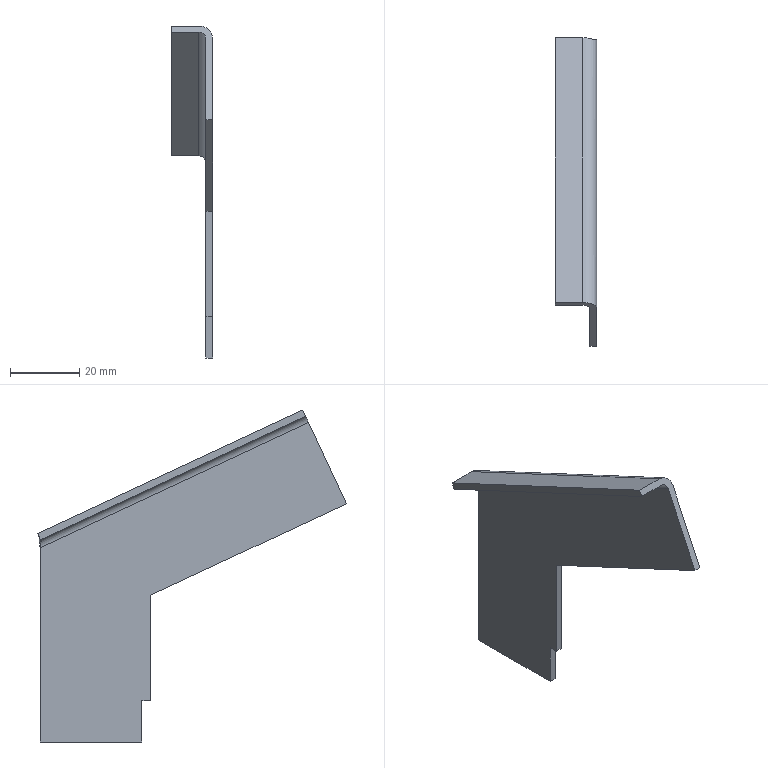Part | NX | features solid 2 | 1 solid | 16 faces | box 12 x 89.507 x 96.207 mm | volume 9121 mm3 | plane 13 | cylinder 2 | spline 1 | commonest cylinder face diameters 4 x1 8 x1
STEP:
#1=CARTESIAN_POINT('',(428.,-1432.5,103.613));
#2=VERTEX_POINT('',#1);
#3=CARTESIAN_POINT('',(428.,-1432.5,115.613));
#4=VERTEX_POINT('',#3);
#5=CARTESIAN_POINT('',(428.,-1432.5,311.243));
#6=DIRECTION('',(0.,0.,1.));
#7=VECTOR('',#6,1000.);
#8=LINE('',#5,#7);
#9=EDGE_CURVE('',#2,#4,#8,.T.);
#10=ORIENTED_EDGE('',*,*,#9,.F.);
#11=CARTESIAN_POINT('',(430.,-1432.5,103.613));
#12=VERTEX_POINT('',#11);
#13=CARTESIAN_POINT('',(430.,-1432.5,103.613));
#14=DIRECTION('',(1.,0.,0.));
#15=VECTOR('',#14,1000.);
#16=LINE('',#13,#15);
#17=EDGE_CURVE('',#2,#12,#16,.T.);
#18=ORIENTED_EDGE('',*,*,#17,.T.);
#19=CARTESIAN_POINT('',(430.,-1432.5,115.613));
#20=VERTEX_POINT('',#19);
#21=CARTESIAN_POINT('',(430.,-1432.5,311.243));
#22=DIRECTION('',(0.,0.,1.));
#23=VECTOR('',#22,1000.);
#24=LINE('',#21,#23);
#25=EDGE_CURVE('',#12,#20,#24,.T.);
#26=ORIENTED_EDGE('',*,*,#25,.T.);
#27=CARTESIAN_POINT('',(430.,-1432.5,115.613));
#28=DIRECTION('',(1.,0.,0.));
#29=VECTOR('',#28,1000.);
#30=LINE('',#27,#29);
#31=EDGE_CURVE('',#4,#20,#30,.T.);
#32=ORIENTED_EDGE('',*,*,#31,.F.);
#33=EDGE_LOOP('',(#10,#18,#26,#32));
#34=FACE_BOUND('',#33,.T.);
#35=CARTESIAN_POINT('',(430.,-1432.5,311.243));
#36=DIRECTION('',(0.,1.,0.));
#37=DIRECTION('',(1.,0.,0.));
#38=AXIS2_PLACEMENT_3D('',#35,#36,#37);
#39=PLANE('',#38);
#40=ADVANCED_FACE('',(#34),#39,.F.);
#41=ORIENTED_EDGE('',*,*,#31,.T.);
#42=CARTESIAN_POINT('',(430.,-1435.,115.613));
#43=VERTEX_POINT('',#42);
#44=CARTESIAN_POINT('',(430.,-1650.,115.613));
#45=DIRECTION('',(0.,-1.,0.));
#46=VECTOR('',#45,1000.);
#47=LINE('',#44,#46);
#48=EDGE_CURVE('',#20,#43,#47,.T.);
#49=ORIENTED_EDGE('',*,*,#48,.T.);
#50=CARTESIAN_POINT('',(428.,-1435.,115.613));
#51=VERTEX_POINT('',#50);
#52=CARTESIAN_POINT('',(430.,-1435.,115.613));
#53=DIRECTION('',(1.,0.,0.));
#54=VECTOR('',#53,1000.);
#55=LINE('',#52,#54);
#56=EDGE_CURVE('',#51,#43,#55,.T.);
#57=ORIENTED_EDGE('',*,*,#56,.F.);
#58=CARTESIAN_POINT('',(428.,-1650.,115.613));
#59=DIRECTION('',(0.,-1.,0.));
#60=VECTOR('',#59,1000.);
#61=LINE('',#58,#60);
#62=EDGE_CURVE('',#4,#51,#61,.T.);
#63=ORIENTED_EDGE('',*,*,#62,.F.);
#64=EDGE_LOOP('',(#41,#49,#57,#63));
#65=FACE_BOUND('',#64,.T.);
#66=CARTESIAN_POINT('',(430.,-1650.,115.613));
#67=DIRECTION('',(0.,0.,1.));
#68=DIRECTION('',(1.,0.,0.));
#69=AXIS2_PLACEMENT_3D('',#66,#67,#68);
#70=PLANE('',#69);
#71=ADVANCED_FACE('',(#65),#70,.F.);
#72=CARTESIAN_POINT('',(428.,-1403.,159.921));
#73=VERTEX_POINT('',#72);
#74=CARTESIAN_POINT('',(428.,-1480.791,196.195));
#75=VERTEX_POINT('',#74);
#76=CARTESIAN_POINT('',(428.,-1403.,159.921));
#77=DIRECTION('',(0.,-0.9063,0.4226));
#78=VECTOR('',#77,1000.);
#79=LINE('',#76,#78);
#80=EDGE_CURVE('',#73,#75,#79,.T.);
#81=ORIENTED_EDGE('',*,*,#80,.T.);
#82=CARTESIAN_POINT('',(426.,-1479.945,198.008));
#83=VERTEX_POINT('',#82);
#84=CARTESIAN_POINT('',(426.,-1480.791,196.195));
#85=DIRECTION('',(0.,-0.9063,0.4226));
#86=DIRECTION('',(0.,0.4226,0.9063));
#87=AXIS2_PLACEMENT_3D('',#84,#85,#86);
#88=CIRCLE('',#87,2.);
#89=EDGE_CURVE('',#75,#83,#88,.T.);
#90=ORIENTED_EDGE('',*,*,#89,.T.);
#91=CARTESIAN_POINT('',(426.,-1403.117,162.182));
#92=VERTEX_POINT('',#91);
#93=CARTESIAN_POINT('',(426.,-1479.945,198.008));
#94=DIRECTION('',(0.,0.9063,-0.4226));
#95=VECTOR('',#94,1000.);
#96=LINE('',#93,#95);
#97=EDGE_CURVE('',#83,#92,#96,.T.);
#98=ORIENTED_EDGE('',*,*,#97,.T.);
#99=CARTESIAN_POINT('',(427.414,-1403.365,161.652));
#100=VERTEX_POINT('',#99);
#101=CARTESIAN_POINT('',(426.,-1403.963,160.37));
#102=DIRECTION('',(0.,-0.9063,0.4226));
#103=DIRECTION('',(1.,0.,0.));
#104=AXIS2_PLACEMENT_3D('',#101,#102,#103);
#105=CIRCLE('',#104,2.);
#106=EDGE_CURVE('',#100,#92,#105,.T.);
#107=ORIENTED_EDGE('',*,*,#106,.F.);
#108=CARTESIAN_POINT('',(427.414,-1403.365,161.652));
#109=CARTESIAN_POINT('',(427.784,-1403.201,161.166));
#110=CARTESIAN_POINT('',(428.,-1403.1,160.545));
#111=CARTESIAN_POINT('',(428.,-1403.,159.921));
#112=B_SPLINE_CURVE_WITH_KNOTS('',3,(#108,#109,#110,#111),.UNSPECIFIED.,.F.,.F.,(4,4),(0.,1.),.UNSPECIFIED.);
#113=EDGE_CURVE('',#100,#73,#112,.T.);
#114=ORIENTED_EDGE('',*,*,#113,.T.);
#115=EDGE_LOOP('',(#81,#90,#98,#107,#114));
#116=FACE_BOUND('',#115,.T.);
#117=CARTESIAN_POINT('',(426.,-1403.,159.921));
#118=DIRECTION('',(0.,-0.9063,0.4226));
#119=DIRECTION('',(-1.,0.,0.));
#120=AXIS2_PLACEMENT_3D('',#117,#118,#119);
#121=CYLINDRICAL_SURFACE('',#120,2.);
#122=ADVANCED_FACE('',(#116),#121,.F.);
#123=CARTESIAN_POINT('',(430.,-1403.,159.921));
#124=VERTEX_POINT('',#123);
#125=CARTESIAN_POINT('',(430.,-1480.791,196.195));
#126=VERTEX_POINT('',#125);
#127=CARTESIAN_POINT('',(430.,-1403.,159.921));
#128=DIRECTION('',(0.,-0.9063,0.4226));
#129=VECTOR('',#128,1000.);
#130=LINE('',#127,#129);
#131=EDGE_CURVE('',#124,#126,#130,.T.);
#132=ORIENTED_EDGE('',*,*,#131,.F.);
#133=CARTESIAN_POINT('',(428.828,-1402.767,162.933));
#134=VERTEX_POINT('',#133);
#135=CARTESIAN_POINT('',(430.,-1403.,159.921));
#136=CARTESIAN_POINT('',(430.,-1402.878,161.02));
#137=CARTESIAN_POINT('',(429.569,-1402.759,162.113));
#138=CARTESIAN_POINT('',(428.828,-1402.767,162.933));
#139=B_SPLINE_CURVE_WITH_KNOTS('',3,(#135,#136,#137,#138),.UNSPECIFIED.,.F.,.F.,(4,4),(0.,1.),.UNSPECIFIED.);
#140=EDGE_CURVE('',#134,#124,#139,.F.);
#141=ORIENTED_EDGE('',*,*,#140,.F.);
#142=CARTESIAN_POINT('',(426.,-1402.272,163.995));
#143=VERTEX_POINT('',#142);
#144=CARTESIAN_POINT('',(426.,-1403.963,160.37));
#145=DIRECTION('',(0.,-0.9063,0.4226));
#146=DIRECTION('',(-1.,0.,0.));
#147=AXIS2_PLACEMENT_3D('',#144,#145,#146);
#148=CIRCLE('',#147,4.);
#149=EDGE_CURVE('',#134,#143,#148,.T.);
#150=ORIENTED_EDGE('',*,*,#149,.T.);
#151=CARTESIAN_POINT('',(426.,-1479.1,199.821));
#152=VERTEX_POINT('',#151);
#153=CARTESIAN_POINT('',(426.,-1479.1,199.821));
#154=DIRECTION('',(0.,0.9063,-0.4226));
#155=VECTOR('',#154,1000.);
#156=LINE('',#153,#155);
#157=EDGE_CURVE('',#152,#143,#156,.T.);
#158=ORIENTED_EDGE('',*,*,#157,.F.);
#159=CARTESIAN_POINT('',(426.,-1480.791,196.195));
#160=DIRECTION('',(0.,-0.9063,0.4226));
#161=DIRECTION('',(-1.,0.,0.));
#162=AXIS2_PLACEMENT_3D('',#159,#160,#161);
#163=CIRCLE('',#162,4.);
#164=EDGE_CURVE('',#126,#152,#163,.T.);
#165=ORIENTED_EDGE('',*,*,#164,.F.);
#166=EDGE_LOOP('',(#132,#141,#150,#158,#165));
#167=FACE_BOUND('',#166,.T.);
#168=CARTESIAN_POINT('',(426.,-1403.,159.921));
#169=DIRECTION('',(0.,-0.9063,0.4226));
#170=DIRECTION('',(-1.,0.,0.));
#171=AXIS2_PLACEMENT_3D('',#168,#169,#170);
#172=CYLINDRICAL_SURFACE('',#171,4.);
#173=ADVANCED_FACE('',(#167),#172,.T.);
#174=ORIENTED_EDGE('',*,*,#113,.F.);
#175=CARTESIAN_POINT('',(428.828,-1402.767,162.933));
#176=DIRECTION('',(0.7071,0.2988,0.6409));
#177=VECTOR('',#176,1000.);
#178=LINE('',#175,#177);
#179=EDGE_CURVE('',#100,#134,#178,.T.);
#180=ORIENTED_EDGE('',*,*,#179,.T.);
#181=ORIENTED_EDGE('',*,*,#140,.T.);
#182=CARTESIAN_POINT('',(428.,-1403.,159.921));
#183=DIRECTION('',(1.,0.,0.));
#184=VECTOR('',#183,1000.);
#185=LINE('',#182,#184);
#186=EDGE_CURVE('',#73,#124,#185,.T.);
#187=ORIENTED_EDGE('',*,*,#186,.F.);
#188=EDGE_LOOP('',(#174,#180,#181,#187));
#189=FACE_BOUND('',#188,.T.);
#190=CARTESIAN_POINT('',(428.828,-1402.767,162.933));
#191=CARTESIAN_POINT('',(429.199,-1402.763,162.523));
#192=CARTESIAN_POINT('',(429.495,-1402.79,162.046));
#193=CARTESIAN_POINT('',(429.896,-1402.878,161.019));
#194=CARTESIAN_POINT('',(430.,-1402.939,160.47));
#195=CARTESIAN_POINT('',(430.,-1403.,159.921));
#196=CARTESIAN_POINT('',(427.414,-1403.365,161.652));
#197=CARTESIAN_POINT('',(427.599,-1403.283,161.409));
#198=CARTESIAN_POINT('',(427.748,-1403.216,161.133));
#199=CARTESIAN_POINT('',(427.948,-1403.1,160.545));
#200=CARTESIAN_POINT('',(428.,-1403.05,160.233));
#201=CARTESIAN_POINT('',(428.,-1403.,159.921));
#202=(BOUNDED_SURFACE()B_SPLINE_SURFACE(1,3,((#190,#191,#192,#193,#194,#195),(#196,#197,#198,#199,#200,#201)),.RULED_SURF.,.F.,.F.,.F.)B_SPLINE_SURFACE_WITH_KNOTS((2,2),(4,2,4),(0.,1.),(0.,0.5,1.),.UNSPECIFIED.)GEOMETRIC_REPRESENTATION_ITEM()RATIONAL_B_SPLINE_SURFACE(((1.,1.,1.,1.,1.,1.),(1.,1.,1.,1.,1.,1.)))REPRESENTATION_ITEM('')SURFACE());
#203=ADVANCED_FACE('',(#189),#202,.F.);
#204=CARTESIAN_POINT('',(418.,-1403.117,162.182));
#205=VERTEX_POINT('',#204);
#206=CARTESIAN_POINT('',(418.,-1479.945,198.008));
#207=VERTEX_POINT('',#206);
#208=CARTESIAN_POINT('',(418.,-1403.117,162.182));
#209=DIRECTION('',(0.,-0.9063,0.4226));
#210=VECTOR('',#209,1000.);
#211=LINE('',#208,#210);
#212=EDGE_CURVE('',#205,#207,#211,.T.);
#213=ORIENTED_EDGE('',*,*,#212,.T.);
#214=CARTESIAN_POINT('',(418.,-1479.1,199.821));
#215=VERTEX_POINT('',#214);
#216=CARTESIAN_POINT('',(418.,-1479.1,199.821));
#217=DIRECTION('',(0.,-0.4226,-0.9063));
#218=VECTOR('',#217,1000.);
#219=LINE('',#216,#218);
#220=EDGE_CURVE('',#215,#207,#219,.T.);
#221=ORIENTED_EDGE('',*,*,#220,.F.);
#222=CARTESIAN_POINT('',(418.,-1402.272,163.995));
#223=VERTEX_POINT('',#222);
#224=CARTESIAN_POINT('',(418.,-1402.272,163.995));
#225=DIRECTION('',(0.,-0.9063,0.4226));
#226=VECTOR('',#225,1000.);
#227=LINE('',#224,#226);
#228=EDGE_CURVE('',#223,#215,#227,.T.);
#229=ORIENTED_EDGE('',*,*,#228,.F.);
#230=CARTESIAN_POINT('',(418.,-1402.272,163.995));
#231=DIRECTION('',(0.,-0.4226,-0.9063));
#232=VECTOR('',#231,1000.);
#233=LINE('',#230,#232);
#234=EDGE_CURVE('',#223,#205,#233,.T.);
#235=ORIENTED_EDGE('',*,*,#234,.T.);
#236=EDGE_LOOP('',(#213,#221,#229,#235));
#237=FACE_BOUND('',#236,.T.);
#238=CARTESIAN_POINT('',(418.,-1402.272,163.995));
#239=DIRECTION('',(1.,0.,0.));
#240=DIRECTION('',(0.,0.,1.));
#241=AXIS2_PLACEMENT_3D('',#238,#239,#240);
#242=PLANE('',#241);
#243=ADVANCED_FACE('',(#237),#242,.F.);
#244=ORIENTED_EDGE('',*,*,#97,.F.);
#245=CARTESIAN_POINT('',(428.278,-1479.945,198.008));
#246=DIRECTION('',(1.,0.,0.));
#247=VECTOR('',#246,1000.);
#248=LINE('',#245,#247);
#249=EDGE_CURVE('',#207,#83,#248,.T.);
#250=ORIENTED_EDGE('',*,*,#249,.F.);
#251=ORIENTED_EDGE('',*,*,#212,.F.);
#252=CARTESIAN_POINT('',(428.278,-1403.117,162.182));
#253=DIRECTION('',(-1.,0.,0.));
#254=VECTOR('',#253,1000.);
#255=LINE('',#252,#254);
#256=EDGE_CURVE('',#92,#205,#255,.T.);
#257=ORIENTED_EDGE('',*,*,#256,.F.);
#258=EDGE_LOOP('',(#244,#250,#251,#257));
#259=FACE_BOUND('',#258,.T.);
#260=CARTESIAN_POINT('',(430.,-1670.659,286.939));
#261=DIRECTION('',(0.,0.4226,0.9063));
#262=DIRECTION('',(1.,0.,0.));
#263=AXIS2_PLACEMENT_3D('',#260,#261,#262);
#264=PLANE('',#263);
#265=ADVANCED_FACE('',(#259),#264,.F.);
#266=CARTESIAN_POINT('',(428.278,-1479.1,199.821));
#267=DIRECTION('',(1.,0.,0.));
#268=VECTOR('',#267,1000.);
#269=LINE('',#266,#268);
#270=EDGE_CURVE('',#215,#152,#269,.T.);
#271=ORIENTED_EDGE('',*,*,#270,.T.);
#272=ORIENTED_EDGE('',*,*,#157,.T.);
#273=CARTESIAN_POINT('',(428.278,-1402.272,163.995));
#274=DIRECTION('',(-1.,0.,0.));
#275=VECTOR('',#274,1000.);
#276=LINE('',#273,#275);
#277=EDGE_CURVE('',#143,#223,#276,.T.);
#278=ORIENTED_EDGE('',*,*,#277,.T.);
#279=ORIENTED_EDGE('',*,*,#228,.T.);
#280=EDGE_LOOP('',(#271,#272,#278,#279));
#281=FACE_BOUND('',#280,.T.);
#282=CARTESIAN_POINT('',(430.,-1669.814,288.752));
#283=DIRECTION('',(0.,0.4226,0.9063));
#284=DIRECTION('',(1.,0.,0.));
#285=AXIS2_PLACEMENT_3D('',#282,#283,#284);
#286=PLANE('',#285);
#287=ADVANCED_FACE('',(#281),#286,.T.);
#288=ORIENTED_EDGE('',*,*,#277,.F.);
#289=ORIENTED_EDGE('',*,*,#149,.F.);
#290=ORIENTED_EDGE('',*,*,#179,.F.);
#291=ORIENTED_EDGE('',*,*,#106,.T.);
#292=ORIENTED_EDGE('',*,*,#256,.T.);
#293=ORIENTED_EDGE('',*,*,#234,.F.);
#294=EDGE_LOOP('',(#288,#289,#290,#291,#292,#293));
#295=FACE_BOUND('',#294,.T.);
#296=CARTESIAN_POINT('',(428.278,-1402.272,163.995));
#297=DIRECTION('',(0.,-0.9063,0.4226));
#298=DIRECTION('',(-1.,0.,0.));
#299=AXIS2_PLACEMENT_3D('',#296,#297,#298);
#300=PLANE('',#299);
#301=ADVANCED_FACE('',(#295),#300,.F.);
#302=ORIENTED_EDGE('',*,*,#9,.T.);
#303=ORIENTED_EDGE('',*,*,#62,.T.);
#304=CARTESIAN_POINT('',(428.,-1435.,146.155));
#305=VERTEX_POINT('',#304);
#306=CARTESIAN_POINT('',(428.,-1435.,123.613));
#307=DIRECTION('',(0.,0.,1.));
#308=VECTOR('',#307,1000.);
#309=LINE('',#306,#308);
#310=EDGE_CURVE('',#51,#305,#309,.T.);
#311=ORIENTED_EDGE('',*,*,#310,.T.);
#312=CARTESIAN_POINT('',(428.,-1491.779,172.631));
#313=VERTEX_POINT('',#312);
#314=CARTESIAN_POINT('',(428.,-1435.,146.155));
#315=DIRECTION('',(0.,-0.9063,0.4226));
#316=VECTOR('',#315,1000.);
#317=LINE('',#314,#316);
#318=EDGE_CURVE('',#305,#313,#317,.T.);
#319=ORIENTED_EDGE('',*,*,#318,.T.);
#320=CARTESIAN_POINT('',(428.,-1491.779,172.631));
#321=DIRECTION('',(0.,0.4226,0.9063));
#322=VECTOR('',#321,1000.);
#323=LINE('',#320,#322);
#324=EDGE_CURVE('',#313,#75,#323,.T.);
#325=ORIENTED_EDGE('',*,*,#324,.T.);
#326=ORIENTED_EDGE('',*,*,#80,.F.);
#327=CARTESIAN_POINT('',(428.,-1403.,103.613));
#328=VERTEX_POINT('',#327);
#329=CARTESIAN_POINT('',(428.,-1403.,123.613));
#330=DIRECTION('',(0.,0.,-1.));
#331=VECTOR('',#330,1000.);
#332=LINE('',#329,#331);
#333=EDGE_CURVE('',#73,#328,#332,.T.);
#334=ORIENTED_EDGE('',*,*,#333,.T.);
#335=CARTESIAN_POINT('',(428.,-1403.,103.613));
#336=DIRECTION('',(0.,-1.,0.));
#337=VECTOR('',#336,1000.);
#338=LINE('',#335,#337);
#339=EDGE_CURVE('',#328,#2,#338,.T.);
#340=ORIENTED_EDGE('',*,*,#339,.T.);
#341=EDGE_LOOP('',(#302,#303,#311,#319,#325,#326,#334,#340));
#342=FACE_BOUND('',#341,.T.);
#343=CARTESIAN_POINT('',(428.,-1650.,331.243));
#344=DIRECTION('',(1.,0.,0.));
#345=DIRECTION('',(0.,0.,1.));
#346=AXIS2_PLACEMENT_3D('',#343,#344,#345);
#347=PLANE('',#346);
#348=ADVANCED_FACE('',(#342),#347,.F.);
#349=CARTESIAN_POINT('',(430.,-1435.,146.155));
#350=VERTEX_POINT('',#349);
#351=CARTESIAN_POINT('',(430.,-1491.779,172.631));
#352=VERTEX_POINT('',#351);
#353=CARTESIAN_POINT('',(430.,-1435.,146.155));
#354=DIRECTION('',(0.,-0.9063,0.4226));
#355=VECTOR('',#354,1000.);
#356=LINE('',#353,#355);
#357=EDGE_CURVE('',#350,#352,#356,.T.);
#358=ORIENTED_EDGE('',*,*,#357,.T.);
#359=CARTESIAN_POINT('',(428.,-1491.779,172.631));
#360=DIRECTION('',(1.,0.,0.));
#361=VECTOR('',#360,1000.);
#362=LINE('',#359,#361);
#363=EDGE_CURVE('',#313,#352,#362,.T.);
#364=ORIENTED_EDGE('',*,*,#363,.F.);
#365=ORIENTED_EDGE('',*,*,#318,.F.);
#366=CARTESIAN_POINT('',(428.,-1435.,146.155));
#367=DIRECTION('',(1.,0.,0.));
#368=VECTOR('',#367,1000.);
#369=LINE('',#366,#368);
#370=EDGE_CURVE('',#305,#350,#369,.T.);
#371=ORIENTED_EDGE('',*,*,#370,.T.);
#372=EDGE_LOOP('',(#358,#364,#365,#371));
#373=FACE_BOUND('',#372,.T.);
#374=CARTESIAN_POINT('',(428.,-1435.,146.155));
#375=DIRECTION('',(0.,0.4226,0.9063));
#376=DIRECTION('',(1.,0.,0.));
#377=AXIS2_PLACEMENT_3D('',#374,#375,#376);
#378=PLANE('',#377);
#379=ADVANCED_FACE('',(#373),#378,.F.);
#380=ORIENTED_EDGE('',*,*,#310,.F.);
#381=ORIENTED_EDGE('',*,*,#56,.T.);
#382=CARTESIAN_POINT('',(430.,-1435.,123.613));
#383=DIRECTION('',(0.,0.,1.));
#384=VECTOR('',#383,1000.);
#385=LINE('',#382,#384);
#386=EDGE_CURVE('',#43,#350,#385,.T.);
#387=ORIENTED_EDGE('',*,*,#386,.T.);
#388=ORIENTED_EDGE('',*,*,#370,.F.);
#389=EDGE_LOOP('',(#380,#381,#387,#388));
#390=FACE_BOUND('',#389,.T.);
#391=CARTESIAN_POINT('',(428.,-1435.,123.613));
#392=DIRECTION('',(0.,1.,0.));
#393=DIRECTION('',(0.,0.,-1.));
#394=AXIS2_PLACEMENT_3D('',#391,#392,#393);
#395=PLANE('',#394);
#396=ADVANCED_FACE('',(#390),#395,.F.);
#397=ORIENTED_EDGE('',*,*,#48,.F.);
#398=ORIENTED_EDGE('',*,*,#25,.F.);
#399=CARTESIAN_POINT('',(430.,-1403.,103.613));
#400=VERTEX_POINT('',#399);
#401=CARTESIAN_POINT('',(430.,-1403.,103.613));
#402=DIRECTION('',(0.,-1.,0.));
#403=VECTOR('',#402,1000.);
#404=LINE('',#401,#403);
#405=EDGE_CURVE('',#400,#12,#404,.T.);
#406=ORIENTED_EDGE('',*,*,#405,.F.);
#407=CARTESIAN_POINT('',(430.,-1403.,123.613));
#408=DIRECTION('',(0.,0.,-1.));
#409=VECTOR('',#408,1000.);
#410=LINE('',#407,#409);
#411=EDGE_CURVE('',#124,#400,#410,.T.);
#412=ORIENTED_EDGE('',*,*,#411,.F.);
#413=ORIENTED_EDGE('',*,*,#131,.T.);
#414=CARTESIAN_POINT('',(430.,-1491.779,172.631));
#415=DIRECTION('',(0.,0.4226,0.9063));
#416=VECTOR('',#415,1000.);
#417=LINE('',#414,#416);
#418=EDGE_CURVE('',#352,#126,#417,.T.);
#419=ORIENTED_EDGE('',*,*,#418,.F.);
#420=ORIENTED_EDGE('',*,*,#357,.F.);
#421=ORIENTED_EDGE('',*,*,#386,.F.);
#422=EDGE_LOOP('',(#397,#398,#406,#412,#413,#419,#420,#421));
#423=FACE_BOUND('',#422,.T.);
#424=CARTESIAN_POINT('',(430.,-1650.,331.243));
#425=DIRECTION('',(1.,0.,0.));
#426=DIRECTION('',(0.,0.,1.));
#427=AXIS2_PLACEMENT_3D('',#424,#425,#426);
#428=PLANE('',#427);
#429=ADVANCED_FACE('',(#423),#428,.T.);
#430=ORIENTED_EDGE('',*,*,#333,.F.);
#431=ORIENTED_EDGE('',*,*,#186,.T.);
#432=ORIENTED_EDGE('',*,*,#411,.T.);
#433=CARTESIAN_POINT('',(428.,-1403.,103.613));
#434=DIRECTION('',(1.,0.,0.));
#435=VECTOR('',#434,1000.);
#436=LINE('',#433,#435);
#437=EDGE_CURVE('',#328,#400,#436,.T.);
#438=ORIENTED_EDGE('',*,*,#437,.F.);
#439=EDGE_LOOP('',(#430,#431,#432,#438));
#440=FACE_BOUND('',#439,.T.);
#441=CARTESIAN_POINT('',(428.,-1403.,123.613));
#442=DIRECTION('',(0.,-1.,0.));
#443=DIRECTION('',(0.,0.,-1.));
#444=AXIS2_PLACEMENT_3D('',#441,#442,#443);
#445=PLANE('',#444);
#446=ADVANCED_FACE('',(#440),#445,.F.);
#447=ORIENTED_EDGE('',*,*,#418,.T.);
#448=ORIENTED_EDGE('',*,*,#164,.T.);
#449=ORIENTED_EDGE('',*,*,#270,.F.);
#450=ORIENTED_EDGE('',*,*,#220,.T.);
#451=ORIENTED_EDGE('',*,*,#249,.T.);
#452=ORIENTED_EDGE('',*,*,#89,.F.);
#453=ORIENTED_EDGE('',*,*,#324,.F.);
#454=ORIENTED_EDGE('',*,*,#363,.T.);
#455=EDGE_LOOP('',(#447,#448,#449,#450,#451,#452,#453,#454));
#456=FACE_BOUND('',#455,.T.);
#457=CARTESIAN_POINT('',(428.,-1491.779,172.631));
#458=DIRECTION('',(0.,0.9063,-0.4226));
#459=DIRECTION('',(-1.,0.,0.));
#460=AXIS2_PLACEMENT_3D('',#457,#458,#459);
#461=PLANE('',#460);
#462=ADVANCED_FACE('',(#456),#461,.F.);
#463=ORIENTED_EDGE('',*,*,#17,.F.);
#464=ORIENTED_EDGE('',*,*,#339,.F.);
#465=ORIENTED_EDGE('',*,*,#437,.T.);
#466=ORIENTED_EDGE('',*,*,#405,.T.);
#467=EDGE_LOOP('',(#463,#464,#465,#466));
#468=FACE_BOUND('',#467,.T.);
#469=CARTESIAN_POINT('',(428.,-1403.,103.613));
#470=DIRECTION('',(0.,0.,1.));
#471=DIRECTION('',(1.,0.,0.));
#472=AXIS2_PLACEMENT_3D('',#469,#470,#471);
#473=PLANE('',#472);
#474=ADVANCED_FACE('',(#468),#473,.F.);
#475=CLOSED_SHELL('',(#40,#71,#122,#173,#203,#243,#265,#287,#301,#348,#379,#396,#429,#446,#462,#474));
#476=MANIFOLD_SOLID_BREP('',#475);
#477=(LENGTH_UNIT()NAMED_UNIT(*)SI_UNIT(.MILLI.,.METRE.));
#478=UNCERTAINTY_MEASURE_WITH_UNIT(LENGTH_MEASURE(0.0508),#477,'','');
#479=(NAMED_UNIT(*)PLANE_ANGLE_UNIT()SI_UNIT($,.RADIAN.));
#480=(NAMED_UNIT(*)SI_UNIT($,.STERADIAN.)SOLID_ANGLE_UNIT());
#481=(GEOMETRIC_REPRESENTATION_CONTEXT(3)GLOBAL_UNCERTAINTY_ASSIGNED_CONTEXT((#478))GLOBAL_UNIT_ASSIGNED_CONTEXT((#477,#479,#480))REPRESENTATION_CONTEXT('',''));
#482=ADVANCED_BREP_SHAPE_REPRESENTATION('',(#476),#481);